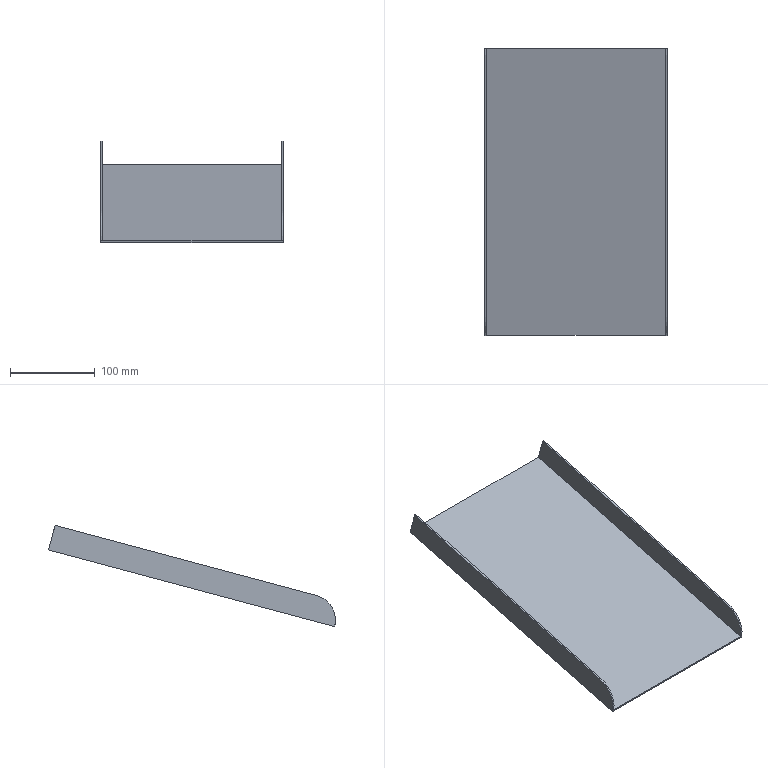Part | NX | features solid 2 | 1 solid | 12 faces | box 215.794 x 339.096 x 119.564 mm | volume 189483 mm3 | plane 10 | cylinder 2 | commonest cylinder face diameters 60 x2
STEP:
#1=CARTESIAN_POINT('',(-797.,-610.733,-523.089));
#2=VERTEX_POINT('',#1);
#3=CARTESIAN_POINT('',(-797.,-948.742,-613.658));
#4=VERTEX_POINT('',#3);
#5=CARTESIAN_POINT('',(-797.,-784.599,-569.676));
#6=DIRECTION('',(0.,-0.9659,-0.2588));
#7=VECTOR('',#6,1000.);
#8=LINE('',#5,#7);
#9=EDGE_CURVE('',#2,#4,#8,.T.);
#10=ORIENTED_EDGE('',*,*,#9,.F.);
#11=CARTESIAN_POINT('',(-1008.794,-610.733,-523.089));
#12=VERTEX_POINT('',#11);
#13=CARTESIAN_POINT('',(-797.,-610.733,-523.089));
#14=DIRECTION('',(1.,0.,0.));
#15=VECTOR('',#14,1000.);
#16=LINE('',#13,#15);
#17=EDGE_CURVE('',#2,#12,#16,.F.);
#18=ORIENTED_EDGE('',*,*,#17,.T.);
#19=CARTESIAN_POINT('',(-1008.794,-948.742,-613.658));
#20=VERTEX_POINT('',#19);
#21=CARTESIAN_POINT('',(-1008.794,-784.599,-569.676));
#22=DIRECTION('',(0.,-0.9659,-0.2588));
#23=VECTOR('',#22,1000.);
#24=LINE('',#21,#23);
#25=EDGE_CURVE('',#12,#20,#24,.T.);
#26=ORIENTED_EDGE('',*,*,#25,.T.);
#27=CARTESIAN_POINT('',(-1010.794,-948.742,-613.658));
#28=VERTEX_POINT('',#27);
#29=CARTESIAN_POINT('',(-1020.794,-948.742,-613.658));
#30=DIRECTION('',(-1.,0.,0.));
#31=VECTOR('',#30,1000.);
#32=LINE('',#29,#31);
#33=EDGE_CURVE('',#28,#20,#32,.F.);
#34=ORIENTED_EDGE('',*,*,#33,.F.);
#35=CARTESIAN_POINT('',(-1010.794,-948.807,-613.675));
#36=VERTEX_POINT('',#35);
#37=CARTESIAN_POINT('',(-1010.794,-784.599,-569.676));
#38=DIRECTION('',(0.,0.9659,0.2588));
#39=VECTOR('',#38,1000.);
#40=LINE('',#37,#39);
#41=EDGE_CURVE('',#28,#36,#40,.F.);
#42=ORIENTED_EDGE('',*,*,#41,.T.);
#43=CARTESIAN_POINT('',(-795.,-948.807,-613.675));
#44=VERTEX_POINT('',#43);
#45=CARTESIAN_POINT('',(-797.,-948.807,-613.675));
#46=DIRECTION('',(1.,0.,0.));
#47=VECTOR('',#46,1000.);
#48=LINE('',#45,#47);
#49=EDGE_CURVE('',#44,#36,#48,.F.);
#50=ORIENTED_EDGE('',*,*,#49,.F.);
#51=CARTESIAN_POINT('',(-795.,-948.742,-613.658));
#52=VERTEX_POINT('',#51);
#53=CARTESIAN_POINT('',(-795.,-784.599,-569.676));
#54=DIRECTION('',(0.,-0.9659,-0.2588));
#55=VECTOR('',#54,1000.);
#56=LINE('',#53,#55);
#57=EDGE_CURVE('',#52,#44,#56,.T.);
#58=ORIENTED_EDGE('',*,*,#57,.F.);
#59=CARTESIAN_POINT('',(-785.,-948.742,-613.658));
#60=DIRECTION('',(1.,0.,0.));
#61=VECTOR('',#60,1000.);
#62=LINE('',#59,#61);
#63=EDGE_CURVE('',#4,#52,#62,.T.);
#64=ORIENTED_EDGE('',*,*,#63,.F.);
#65=EDGE_LOOP('',(#10,#18,#26,#34,#42,#50,#58,#64));
#66=FACE_BOUND('',#65,.T.);
#67=CARTESIAN_POINT('',(-797.,-784.599,-569.676));
#68=DIRECTION('',(0.,-0.2588,0.9659));
#69=DIRECTION('',(1.,0.,0.));
#70=AXIS2_PLACEMENT_3D('',#67,#68,#69);
#71=PLANE('',#70);
#72=ADVANCED_FACE('',(#66),#71,.T.);
#73=ORIENTED_EDGE('',*,*,#17,.F.);
#74=CARTESIAN_POINT('',(-797.,-617.98,-496.043));
#75=VERTEX_POINT('',#74);
#76=CARTESIAN_POINT('',(-797.,-610.215,-525.021));
#77=DIRECTION('',(0.,0.2588,-0.9659));
#78=VECTOR('',#77,1000.);
#79=LINE('',#76,#78);
#80=EDGE_CURVE('',#2,#75,#79,.F.);
#81=ORIENTED_EDGE('',*,*,#80,.T.);
#82=CARTESIAN_POINT('',(-795.,-617.98,-496.043));
#83=VERTEX_POINT('',#82);
#84=CARTESIAN_POINT('',(-797.,-617.98,-496.043));
#85=DIRECTION('',(-1.,0.,0.));
#86=VECTOR('',#85,1000.);
#87=LINE('',#84,#86);
#88=EDGE_CURVE('',#83,#75,#87,.T.);
#89=ORIENTED_EDGE('',*,*,#88,.F.);
#90=CARTESIAN_POINT('',(-795.,-610.215,-525.021));
#91=VERTEX_POINT('',#90);
#92=CARTESIAN_POINT('',(-795.,-610.215,-525.021));
#93=DIRECTION('',(0.,0.2588,-0.9659));
#94=VECTOR('',#93,1000.);
#95=LINE('',#92,#94);
#96=EDGE_CURVE('',#91,#83,#95,.F.);
#97=ORIENTED_EDGE('',*,*,#96,.F.);
#98=CARTESIAN_POINT('',(-1010.794,-610.215,-525.021));
#99=VERTEX_POINT('',#98);
#100=CARTESIAN_POINT('',(-797.,-610.215,-525.021));
#101=DIRECTION('',(1.,0.,0.));
#102=VECTOR('',#101,1000.);
#103=LINE('',#100,#102);
#104=EDGE_CURVE('',#91,#99,#103,.F.);
#105=ORIENTED_EDGE('',*,*,#104,.T.);
#106=CARTESIAN_POINT('',(-1010.794,-617.98,-496.043));
#107=VERTEX_POINT('',#106);
#108=CARTESIAN_POINT('',(-1010.794,-610.215,-525.021));
#109=DIRECTION('',(0.,-0.2588,0.9659));
#110=VECTOR('',#109,1000.);
#111=LINE('',#108,#110);
#112=EDGE_CURVE('',#99,#107,#111,.T.);
#113=ORIENTED_EDGE('',*,*,#112,.T.);
#114=CARTESIAN_POINT('',(-1008.794,-617.98,-496.043));
#115=VERTEX_POINT('',#114);
#116=CARTESIAN_POINT('',(-797.,-617.98,-496.043));
#117=DIRECTION('',(-1.,0.,0.));
#118=VECTOR('',#117,1000.);
#119=LINE('',#116,#118);
#120=EDGE_CURVE('',#107,#115,#119,.F.);
#121=ORIENTED_EDGE('',*,*,#120,.T.);
#122=CARTESIAN_POINT('',(-1008.794,-610.215,-525.021));
#123=DIRECTION('',(0.,0.2588,-0.9659));
#124=VECTOR('',#123,1000.);
#125=LINE('',#122,#124);
#126=EDGE_CURVE('',#12,#115,#125,.F.);
#127=ORIENTED_EDGE('',*,*,#126,.F.);
#128=EDGE_LOOP('',(#73,#81,#89,#97,#105,#113,#121,#127));
#129=FACE_BOUND('',#128,.T.);
#130=CARTESIAN_POINT('',(-797.,-610.215,-525.021));
#131=DIRECTION('',(0.,0.9659,0.2588));
#132=DIRECTION('',(-1.,0.,0.));
#133=AXIS2_PLACEMENT_3D('',#130,#131,#132);
#134=PLANE('',#133);
#135=ADVANCED_FACE('',(#129),#134,.T.);
#136=CARTESIAN_POINT('',(-795.,-948.289,-615.607));
#137=VERTEX_POINT('',#136);
#138=CARTESIAN_POINT('',(-795.,-948.289,-615.607));
#139=DIRECTION('',(0.,-0.2588,0.9659));
#140=VECTOR('',#139,1000.);
#141=LINE('',#138,#140);
#142=EDGE_CURVE('',#137,#44,#141,.T.);
#143=ORIENTED_EDGE('',*,*,#142,.F.);
#144=CARTESIAN_POINT('',(-795.,-784.082,-571.608));
#145=DIRECTION('',(0.,-0.9659,-0.2588));
#146=VECTOR('',#145,1000.);
#147=LINE('',#144,#146);
#148=EDGE_CURVE('',#91,#137,#147,.T.);
#149=ORIENTED_EDGE('',*,*,#148,.F.);
#150=ORIENTED_EDGE('',*,*,#96,.T.);
#151=CARTESIAN_POINT('',(-795.,-927.076,-578.865));
#152=VERTEX_POINT('',#151);
#153=CARTESIAN_POINT('',(-795.,-791.846,-542.63));
#154=DIRECTION('',(0.,0.9659,0.2588));
#155=VECTOR('',#154,1000.);
#156=LINE('',#153,#155);
#157=EDGE_CURVE('',#83,#152,#156,.F.);
#158=ORIENTED_EDGE('',*,*,#157,.T.);
#159=CARTESIAN_POINT('',(-795.,-919.311,-607.843));
#160=DIRECTION('',(-1.,0.,0.));
#161=DIRECTION('',(0.,0.,1.));
#162=AXIS2_PLACEMENT_3D('',#159,#160,#161);
#163=CIRCLE('',#162,30.);
#164=EDGE_CURVE('',#152,#52,#163,.F.);
#165=ORIENTED_EDGE('',*,*,#164,.T.);
#166=ORIENTED_EDGE('',*,*,#57,.T.);
#167=EDGE_LOOP('',(#143,#149,#150,#158,#165,#166));
#168=FACE_BOUND('',#167,.T.);
#169=CARTESIAN_POINT('',(-795.,-784.082,-571.608));
#170=DIRECTION('',(-1.,0.,0.));
#171=DIRECTION('',(0.,-0.9659,-0.2588));
#172=AXIS2_PLACEMENT_3D('',#169,#170,#171);
#173=PLANE('',#172);
#174=ADVANCED_FACE('',(#168),#173,.F.);
#175=ORIENTED_EDGE('',*,*,#142,.T.);
#176=ORIENTED_EDGE('',*,*,#49,.T.);
#177=CARTESIAN_POINT('',(-1010.794,-948.289,-615.607));
#178=VERTEX_POINT('',#177);
#179=CARTESIAN_POINT('',(-1010.794,-948.289,-615.607));
#180=DIRECTION('',(0.,0.2588,-0.9659));
#181=VECTOR('',#180,1000.);
#182=LINE('',#179,#181);
#183=EDGE_CURVE('',#178,#36,#182,.F.);
#184=ORIENTED_EDGE('',*,*,#183,.F.);
#185=CARTESIAN_POINT('',(-797.,-948.289,-615.607));
#186=DIRECTION('',(-1.,0.,0.));
#187=VECTOR('',#186,1000.);
#188=LINE('',#185,#187);
#189=EDGE_CURVE('',#137,#178,#188,.T.);
#190=ORIENTED_EDGE('',*,*,#189,.F.);
#191=EDGE_LOOP('',(#175,#176,#184,#190));
#192=FACE_BOUND('',#191,.T.);
#193=CARTESIAN_POINT('',(-797.,-948.289,-615.607));
#194=DIRECTION('',(0.,0.9659,0.2588));
#195=DIRECTION('',(-1.,0.,0.));
#196=AXIS2_PLACEMENT_3D('',#193,#194,#195);
#197=PLANE('',#196);
#198=ADVANCED_FACE('',(#192),#197,.F.);
#199=ORIENTED_EDGE('',*,*,#41,.F.);
#200=CARTESIAN_POINT('',(-1010.794,-927.076,-578.865));
#201=VERTEX_POINT('',#200);
#202=CARTESIAN_POINT('',(-1010.794,-919.311,-607.843));
#203=DIRECTION('',(-1.,0.,0.));
#204=DIRECTION('',(0.,0.,1.));
#205=AXIS2_PLACEMENT_3D('',#202,#203,#204);
#206=CIRCLE('',#205,30.);
#207=EDGE_CURVE('',#28,#201,#206,.T.);
#208=ORIENTED_EDGE('',*,*,#207,.T.);
#209=CARTESIAN_POINT('',(-1010.794,-791.846,-542.63));
#210=DIRECTION('',(0.,0.9659,0.2588));
#211=VECTOR('',#210,1000.);
#212=LINE('',#209,#211);
#213=EDGE_CURVE('',#107,#201,#212,.F.);
#214=ORIENTED_EDGE('',*,*,#213,.F.);
#215=ORIENTED_EDGE('',*,*,#112,.F.);
#216=CARTESIAN_POINT('',(-1010.794,-784.082,-571.608));
#217=DIRECTION('',(0.,0.9659,0.2588));
#218=VECTOR('',#217,1000.);
#219=LINE('',#216,#218);
#220=EDGE_CURVE('',#99,#178,#219,.F.);
#221=ORIENTED_EDGE('',*,*,#220,.T.);
#222=ORIENTED_EDGE('',*,*,#183,.T.);
#223=EDGE_LOOP('',(#199,#208,#214,#215,#221,#222));
#224=FACE_BOUND('',#223,.T.);
#225=CARTESIAN_POINT('',(-1010.794,-784.082,-571.608));
#226=DIRECTION('',(-1.,0.,0.));
#227=DIRECTION('',(0.,-0.9659,-0.2588));
#228=AXIS2_PLACEMENT_3D('',#225,#226,#227);
#229=PLANE('',#228);
#230=ADVANCED_FACE('',(#224),#229,.T.);
#231=ORIENTED_EDGE('',*,*,#220,.F.);
#232=ORIENTED_EDGE('',*,*,#104,.F.);
#233=ORIENTED_EDGE('',*,*,#148,.T.);
#234=ORIENTED_EDGE('',*,*,#189,.T.);
#235=EDGE_LOOP('',(#231,#232,#233,#234));
#236=FACE_BOUND('',#235,.T.);
#237=CARTESIAN_POINT('',(-797.,-784.082,-571.608));
#238=DIRECTION('',(0.,-0.2588,0.9659));
#239=DIRECTION('',(1.,0.,0.));
#240=AXIS2_PLACEMENT_3D('',#237,#238,#239);
#241=PLANE('',#240);
#242=ADVANCED_FACE('',(#236),#241,.F.);
#243=ORIENTED_EDGE('',*,*,#213,.T.);
#244=CARTESIAN_POINT('',(-1008.794,-927.076,-578.865));
#245=VERTEX_POINT('',#244);
#246=CARTESIAN_POINT('',(-1020.794,-927.076,-578.865));
#247=DIRECTION('',(-1.,0.,0.));
#248=VECTOR('',#247,1000.);
#249=LINE('',#246,#248);
#250=EDGE_CURVE('',#201,#245,#249,.F.);
#251=ORIENTED_EDGE('',*,*,#250,.T.);
#252=CARTESIAN_POINT('',(-1008.794,-791.846,-542.63));
#253=DIRECTION('',(0.,-0.9659,-0.2588));
#254=VECTOR('',#253,1000.);
#255=LINE('',#252,#254);
#256=EDGE_CURVE('',#115,#245,#255,.T.);
#257=ORIENTED_EDGE('',*,*,#256,.F.);
#258=ORIENTED_EDGE('',*,*,#120,.F.);
#259=EDGE_LOOP('',(#243,#251,#257,#258));
#260=FACE_BOUND('',#259,.T.);
#261=CARTESIAN_POINT('',(-1020.794,-791.846,-542.63));
#262=DIRECTION('',(0.,0.2588,-0.9659));
#263=DIRECTION('',(0.,-0.9659,-0.2588));
#264=AXIS2_PLACEMENT_3D('',#261,#262,#263);
#265=PLANE('',#264);
#266=ADVANCED_FACE('',(#260),#265,.F.);
#267=ORIENTED_EDGE('',*,*,#25,.F.);
#268=ORIENTED_EDGE('',*,*,#126,.T.);
#269=ORIENTED_EDGE('',*,*,#256,.T.);
#270=CARTESIAN_POINT('',(-1008.794,-919.311,-607.843));
#271=DIRECTION('',(-1.,0.,0.));
#272=DIRECTION('',(0.,0.,1.));
#273=AXIS2_PLACEMENT_3D('',#270,#271,#272);
#274=CIRCLE('',#273,30.);
#275=EDGE_CURVE('',#245,#20,#274,.F.);
#276=ORIENTED_EDGE('',*,*,#275,.T.);
#277=EDGE_LOOP('',(#267,#268,#269,#276));
#278=FACE_BOUND('',#277,.T.);
#279=CARTESIAN_POINT('',(-1008.794,-784.082,-571.608));
#280=DIRECTION('',(-1.,0.,0.));
#281=DIRECTION('',(0.,-0.2588,0.9659));
#282=AXIS2_PLACEMENT_3D('',#279,#280,#281);
#283=PLANE('',#282);
#284=ADVANCED_FACE('',(#278),#283,.F.);
#285=ORIENTED_EDGE('',*,*,#207,.F.);
#286=ORIENTED_EDGE('',*,*,#33,.T.);
#287=ORIENTED_EDGE('',*,*,#275,.F.);
#288=ORIENTED_EDGE('',*,*,#250,.F.);
#289=EDGE_LOOP('',(#285,#286,#287,#288));
#290=FACE_BOUND('',#289,.T.);
#291=CARTESIAN_POINT('',(-1020.794,-919.311,-607.843));
#292=DIRECTION('',(-1.,0.,0.));
#293=DIRECTION('',(0.,-0.2588,0.9659));
#294=AXIS2_PLACEMENT_3D('',#291,#292,#293);
#295=CYLINDRICAL_SURFACE('',#294,30.);
#296=ADVANCED_FACE('',(#290),#295,.T.);
#297=CARTESIAN_POINT('',(-797.,-927.076,-578.865));
#298=VERTEX_POINT('',#297);
#299=CARTESIAN_POINT('',(-797.,-791.846,-542.63));
#300=DIRECTION('',(0.,0.9659,0.2588));
#301=VECTOR('',#300,1000.);
#302=LINE('',#299,#301);
#303=EDGE_CURVE('',#75,#298,#302,.F.);
#304=ORIENTED_EDGE('',*,*,#303,.T.);
#305=CARTESIAN_POINT('',(-785.,-927.076,-578.865));
#306=DIRECTION('',(-1.,0.,0.));
#307=VECTOR('',#306,1000.);
#308=LINE('',#305,#307);
#309=EDGE_CURVE('',#298,#152,#308,.F.);
#310=ORIENTED_EDGE('',*,*,#309,.T.);
#311=ORIENTED_EDGE('',*,*,#157,.F.);
#312=ORIENTED_EDGE('',*,*,#88,.T.);
#313=EDGE_LOOP('',(#304,#310,#311,#312));
#314=FACE_BOUND('',#313,.T.);
#315=CARTESIAN_POINT('',(-785.,-791.846,-542.63));
#316=DIRECTION('',(0.,0.2588,-0.9659));
#317=DIRECTION('',(0.,-0.9659,-0.2588));
#318=AXIS2_PLACEMENT_3D('',#315,#316,#317);
#319=PLANE('',#318);
#320=ADVANCED_FACE('',(#314),#319,.F.);
#321=ORIENTED_EDGE('',*,*,#80,.F.);
#322=ORIENTED_EDGE('',*,*,#9,.T.);
#323=CARTESIAN_POINT('',(-797.,-919.311,-607.843));
#324=DIRECTION('',(-1.,0.,0.));
#325=DIRECTION('',(0.,0.,1.));
#326=AXIS2_PLACEMENT_3D('',#323,#324,#325);
#327=CIRCLE('',#326,30.);
#328=EDGE_CURVE('',#4,#298,#327,.T.);
#329=ORIENTED_EDGE('',*,*,#328,.T.);
#330=ORIENTED_EDGE('',*,*,#303,.F.);
#331=EDGE_LOOP('',(#321,#322,#329,#330));
#332=FACE_BOUND('',#331,.T.);
#333=CARTESIAN_POINT('',(-797.,-784.082,-571.608));
#334=DIRECTION('',(-1.,0.,0.));
#335=DIRECTION('',(0.,-0.2588,0.9659));
#336=AXIS2_PLACEMENT_3D('',#333,#334,#335);
#337=PLANE('',#336);
#338=ADVANCED_FACE('',(#332),#337,.T.);
#339=ORIENTED_EDGE('',*,*,#328,.F.);
#340=ORIENTED_EDGE('',*,*,#63,.T.);
#341=ORIENTED_EDGE('',*,*,#164,.F.);
#342=ORIENTED_EDGE('',*,*,#309,.F.);
#343=EDGE_LOOP('',(#339,#340,#341,#342));
#344=FACE_BOUND('',#343,.T.);
#345=CARTESIAN_POINT('',(-785.,-919.311,-607.843));
#346=DIRECTION('',(1.,0.,0.));
#347=DIRECTION('',(0.,0.2588,-0.9659));
#348=AXIS2_PLACEMENT_3D('',#345,#346,#347);
#349=CYLINDRICAL_SURFACE('',#348,30.);
#350=ADVANCED_FACE('',(#344),#349,.T.);
#351=CLOSED_SHELL('',(#72,#135,#174,#198,#230,#242,#266,#284,#296,#320,#338,#350));
#352=MANIFOLD_SOLID_BREP('',#351);
#353=(LENGTH_UNIT()NAMED_UNIT(*)SI_UNIT(.MILLI.,.METRE.));
#354=UNCERTAINTY_MEASURE_WITH_UNIT(LENGTH_MEASURE(0.00001),#353,'','');
#355=(NAMED_UNIT(*)PLANE_ANGLE_UNIT()SI_UNIT($,.RADIAN.));
#356=(NAMED_UNIT(*)SI_UNIT($,.STERADIAN.)SOLID_ANGLE_UNIT());
#357=(GEOMETRIC_REPRESENTATION_CONTEXT(3)GLOBAL_UNCERTAINTY_ASSIGNED_CONTEXT((#354))GLOBAL_UNIT_ASSIGNED_CONTEXT((#353,#355,#356))REPRESENTATION_CONTEXT('',''));
#358=ADVANCED_BREP_SHAPE_REPRESENTATION('',(#352),#357);